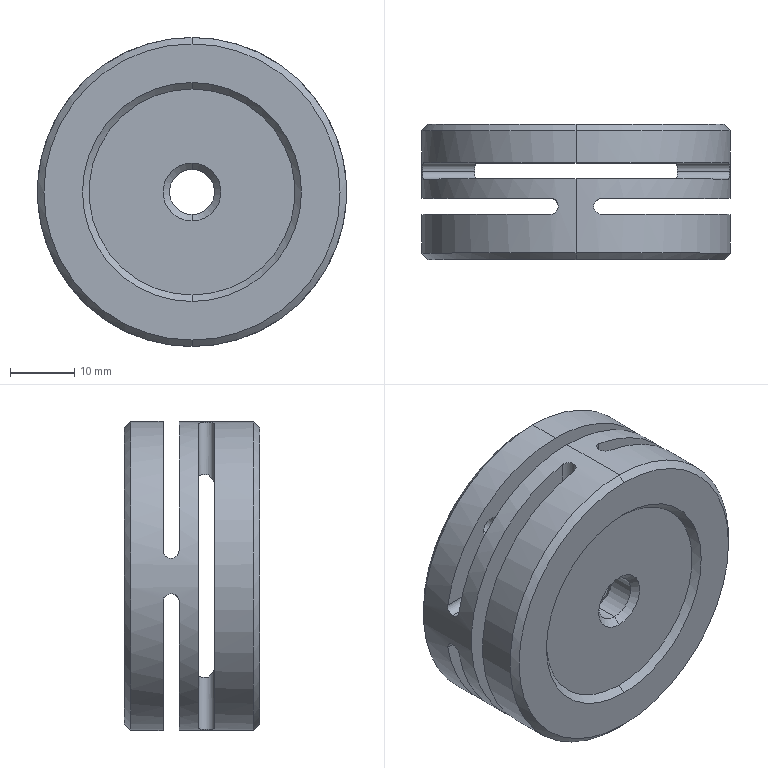Part | SolidWorks | features ICE 3, Chamfer 1, Extrusion 1, HoleWzd 1 | 1 solid | 67 faces | box 48 x 21 x 48 mm | volume 20684 mm3 | cone 31 | cylinder 26 | plane 10 | commonest cylinder face diameters 2.5 x12 3.3 x8 7 x2 32 x2 48 x2